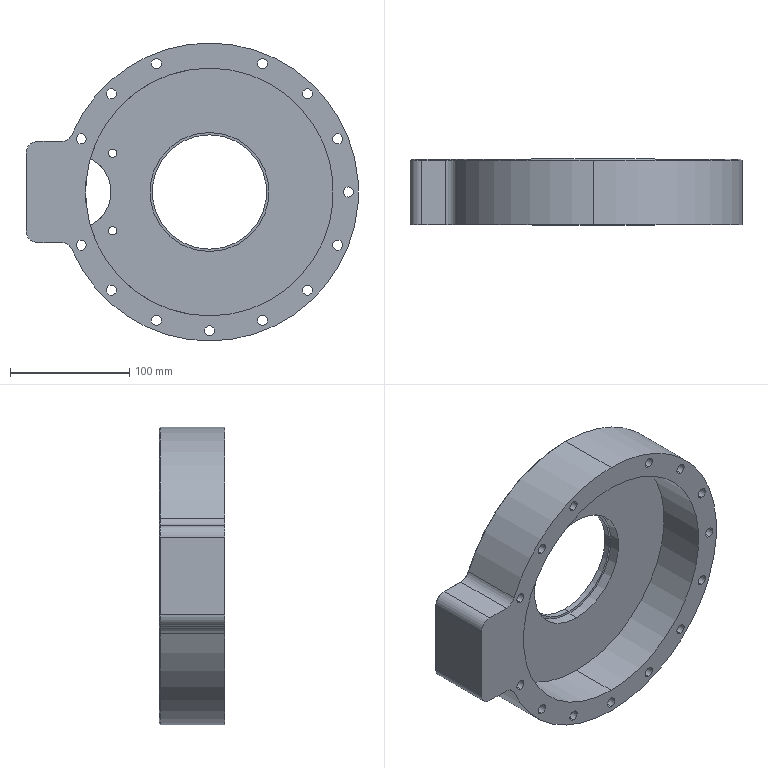Part | SolidWorks | features HoleWzd 2, ICE 2, Chamfer 1, Fillet 1, Revolution 1 | 1 solid | 73 faces | box 279 x 55 x 250 mm | volume 1187209 mm3 | cylinder 51 | cone 11 | plane 11 | commonest cylinder face diameters 8.5 x28 6.8 x8 20 x4 250 x3 62.5 x2 96 x2